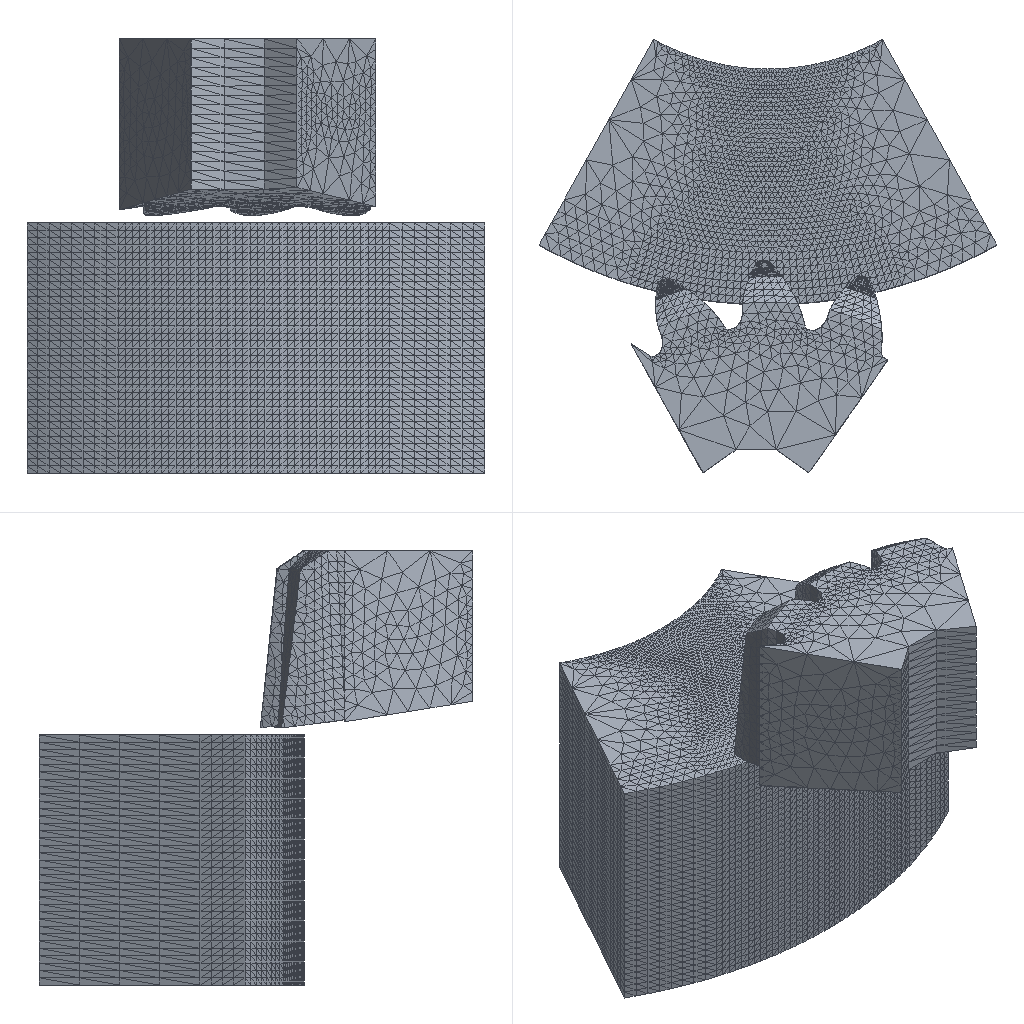Simulation study | abaqus
Set-up summary:
category,name,step,type,value,unit,region
solver,abaqus
solver,version,,,Abaqus/Explicit 3DEXPERIENCE R2017x
units,not stated in the deck,,not stated
analysis,deck,,dynamic temperature-displacement,dynamic temperature-displacement
load_step,Step-1,Step-1,dynamic temperature-displacement
load_step,requested,,,1
mesh,nodes,,,32609
mesh,elements,,,169036
element_type,C3D4T,,solid,169036
load,load commands in deck,,count,2
bc,support commands in deck,,count,9
material,TOOL,,in results
material,WORK,,in results
check,setup vs results,,match,"per instance, exact: element labels, types and connectivity; labels of the nodes the elements use; coordinates of those nodes at SINGLE_PRECISION in 2 of 2 instance(s)"
Abaqus input file, long lists of numbers shortened:
*Heading
** Job name: Job-1 Model name: Model-1
** Generated by: Abaqus/CAE 2017
*Preprint, echo=NO, model=NO, history=NO, contact=NO
**
** PARTS
**
*Part, name=chilun
*Node
      1,  -7.776,  -13.983,           0.
      2,   7.776,  -13.983,           0.
** (28105 more lines like these left out)
*Element, type=C3D4T
     1,  7239,  7240,  7241,  7242
     2,  7239,  7243,  7244,  7245
** (147323 more lines like these left out)
*Nset, nset=Set-1, generate
     1,  28107,      1
*Elset, elset=Set-1, generate
      1,  147325,       1
*Nset, nset=T-workwork, generate
     1,  28107,      1
*Nset, nset=chipchip
   229,   285,   286,   432,   433,   434,   435,   436,   437,   438,   439,   440,   441,   442,   443,   444
   445,   446,   447,   448,   449,   450,   451,   452,   453,   454,   455,   456,   457,   458,   459,   460
** (415 more lines like these left out)
*Nset, nset=chipCHIPCHIP
     7,     8,    12,    13,    16,    17,    18,   226,   227,   228,   229,   230,   231,   232,   247,   284
   285,   286,   287,   288,   289,   312,   313,   314,   315,   316,   317,   318,   319,   320,   321,   322
** (599 more lines like these left out)
** Section: work
*Solid Section, elset=Set-1, material=work
,
*End Part
**
*Part, name=tool
*Node
      1,   6.879,   18.78,           0.
      2,   6.196,   19.016,           0.
** (4500 more lines like these left out)
*Element, type=C3D4T
    1, 1736, 1737, 1738, 1739
    2, 1736, 1737, 1740, 1741
** (21709 more lines like these left out)
*Nset, nset=Set-1, generate
    1,  4502,     1
*Elset, elset=Set-1, generate
     1,  21711,      1
*Nset, nset=T-tool, generate
    1,  4502,     1
*Elset, elset=rigid, generate
     1,  21711,      1
*Elset, elset=_Surf-TOOL_S1, internal
   289,  2480,  2654,  2749,  3263,  3421,  3537,  4059,  4278,  4377,  4379,  4526,  4713,  4939,  5089,  5099
  5112,  5163,  5165,  5179,  5310,  5360,  5422,  5425,  5432,  5519,  5599,  5829,  5840,  5844,  5858,  5898
** (9 more lines like these left out)
*Elset, elset=_Surf-TOOL_S2, internal
    20,  2561,  2716,  2718,  2722,  2865,  3162,  3194,  3410,  3693,  3888,  3892,  3899,  4051,  4112,  4175
  4184,  4216,  4263,  4300,  4427,  4482,  4558,  4581,  4692,  5039,  5047,  5050,  5070,  5095,  5107,  5224
** (12 more lines like these left out)
*Elset, elset=_Surf-TOOL_S3, internal
    30,   138,   161,   173,   181,   278,   284,   289,   298,   338,   342,   349,   386,   437,   443,   453
   517,   567,   604,   608,   693,   773,   776,   860,  1021,  1053,  1105,  1109,  1162,  1191,  1202,  1211
** (179 more lines like these left out)
*Elset, elset=_Surf-TOOL_S4, internal
    21,   332,   340,   370,   433,   441,  2045,  2447,  2475,  2636,  2637,  2645,  2718,  2739,  2861,  3141
  3224,  3443,  3488,  3490,  3680,  4059,  4316,  4380,  4399,  4532,  4582,  4590,  4685,  4687,  4816,  4924
** (10 more lines like these left out)
*Surface, type=ELEMENT, name=Surf-TOOL
_Surf-TOOL_S1, S1
_Surf-TOOL_S2, S2
_Surf-TOOL_S4, S4
_Surf-TOOL_S3, S3
** Section: tool
*Solid Section, elset=Set-1, material=tool
,
*End Part
**
**
** ASSEMBLY
**
*Assembly, name=Assembly
**
*Instance, name=tool, part=tool
24.72, -0.1302, 38.047
*End Instance
**
*Instance, name=chilun, part=chilun
24.72, 48.87, 37.547
*End Instance
**
*Node
      1,   23.911,   7.188,   50.047
*Node
      2,   24.72, -0.1305,   38.047
*Nset, nset=RP-1
 1,
*Nset, nset=Set-3, instance=chilun
    3,    4,    5,    7,   15,   16,  104,  105,  106,  107,  108,  109,  110,  111,  112,  113
  114,  115,  116,  117,  118,  119,  120,  121,  122,  123,  124,  125,  126,  127,  128,  129
** (80 more lines like these left out)
*Elset, elset=Set-3, instance=chilun
    997,   1831,   2493,   2694,   4756,   6910,   9249,   9879,  10099,  10165,  10171,  10176,  10180,  10231,  10244,  10249
  10285,  10296,  10625,  10641,  10645,  10669,  10679,  10705,  10706,  10711,  10714,  10718,  10735,  10744,  10752,  10758
** (154 more lines like these left out)
*Nset, nset=Set-4, instance=chilun
    1,    2,    3,    4,   21,   22,   23,   24,   25,   26,   27,   28,   29,   30,   31,   32
   33,   34,   35,   36,   37,   38,   39,   40,   41,   42,   43,   44,   45,   46,   47,   48
** (112 more lines like these left out)
*Elset, elset=Set-4, instance=chilun
     94,     99,    116,    562,    573,    609,    678,    803,   1447,   1737,   1800,   1839,   1851,   2027,   2249,   2348
   2516,   2687,   2879,   2903,   2921,   3046,   4125,   4962,   5161,   5242,   5928,   6371,   6404,   7096,   7967,   8669
** (215 more lines like these left out)
*Nset, nset=Set-5
 2,
*Nset, nset=_PickedSet10, internal
 2,
*Surface, type=NODE, name=chilun_chipCHIPCHIP_CNS_, internal
chilun.chipCHIPCHIP, 1.
** Constraint: Constraint-1
*Rigid Body, ref node=_PickedSet10, elset=tool.rigid
*End Assembly
**
** MATERIALS
**
*Material, name=tool
*Conductivity
17.,
*Density
 7.84e-09,
*Elastic
210000., 0.3
*Inelastic Heat Fraction
         0.9,
*Specific Heat
 4.18e+08,
*Material, name=work
*Conductivity
52.,
*Damage Initiation, criterion=JOHNSON COOK
 -0.09,  0.27, -0.48, 0.014,  3.87, 1000.,   25.,    1.
*Damage Evolution, type=DISPLACEMENT
 0.003,
*Density
 7.85e-09,
*Elastic
226000., 0.28
*Expansion
 1.2e-05,
*Inelastic Heat Fraction
         0.9,
*Plastic, hardening=JOHNSON COOK
1112.,1063.,  0.2, 0.62,1000.,  25.
*Rate Dependent, type=JOHNSON COOK
 0.01,1.
*Specific Heat
 4.7e+08,
**
** INTERACTION PROPERTIES
**
*Surface Interaction, name=IntProp-1
*Friction
 0.3,
*Surface Behavior, pressure-overclosure=HARD
*Gap Heat Generation
1., 0.5
**
** BOUNDARY CONDITIONS
**
** Name: BC-2 Type: 对称/反对称/完全固定
*Boundary
Set-3, ZSYMM
** Name: BC-3 Type: 位移/转角
*Boundary
Set-4, 1, 1
Set-4, 2, 2
**
** PREDEFINED FIELDS
**
** Name: Predefined Field-1   Type: Temperature
*Initial Conditions, type=TEMPERATURE
chilun.T-workwork, 20.
** Name: Predefined Field-2   Type: Temperature
*Initial Conditions, type=TEMPERATURE
tool.T-tool, 20.
** ----------------------------------------------------------------
**
** STEP: Step-1
**
*Step, name=Step-1, nlgeom=YES
*Dynamic Temperature-displacement, Explicit
, 1.
*Bulk Viscosity
0.06, 1.2
** Mass Scaling: Semi-Automatic
**               Whole Model
*Fixed Mass Scaling, factor=200.
**
** BOUNDARY CONDITIONS
**
** Name: qiexue Type: velocity/angular velocity
*Boundary, type=VELOCITY
Set-5, 1, 1
Set-5, 2, 2
Set-5, 3, 3, -412.6
Set-5, 4, 4
Set-5, 5, 5
Set-5, 6, 6, 0.1447
**
** INTERACTIONS
**
** Interaction: Int-1
*Contact Pair, interaction=IntProp-1, mechanical constraint=KINEMATIC, cpset=Int-1
tool.Surf-TOOL, chilun_chipCHIPCHIP_CNS_
**
** OUTPUT REQUESTS
**
*Restart, write, number interval=1, time marks=NO
**
** FIELD OUTPUT: F-Output-1
**
*Output, field, number interval=100
*Node Output
NT, RF, U, V
*Element Output, directions=YES
MISES, PE, PEEQ, S, STATUS, TEMP
*Output, history, frequency=0
*End Step
Results summary:
result,step,Step-1,partial,increments=1 time=0.0/1.0
result,analysis,,,"dynamic temperature-displacement, explict"
result,last_loadstep,,,1
result,primary field,,,"U, NT11"
result,reaction total,,FX,1.5e-05,model units
result,reaction total,,FY,-0.000681,model units
result,reaction total,,FZ,0.0,model units